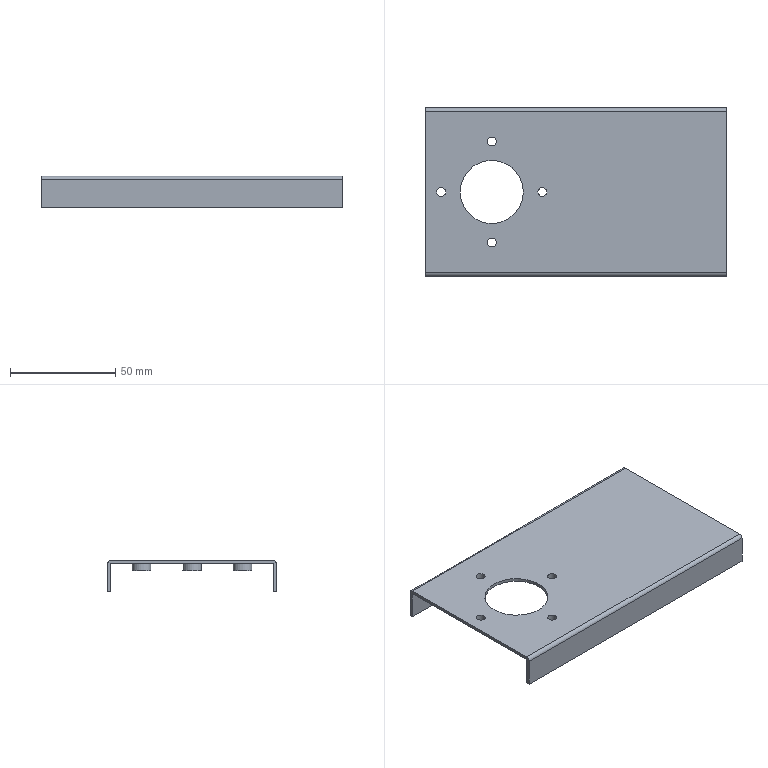Part | STEP file | FHD-021-001-X rack welded part X | 1 solid | 27 faces | box 143 x 80 x 15 mm | volume 22271 mm3 | plane 14 | cylinder 13 | commonest cylinder face diameters 4.2 x4 8.7 x4 0.4 x2 3.4 x2 30 x1